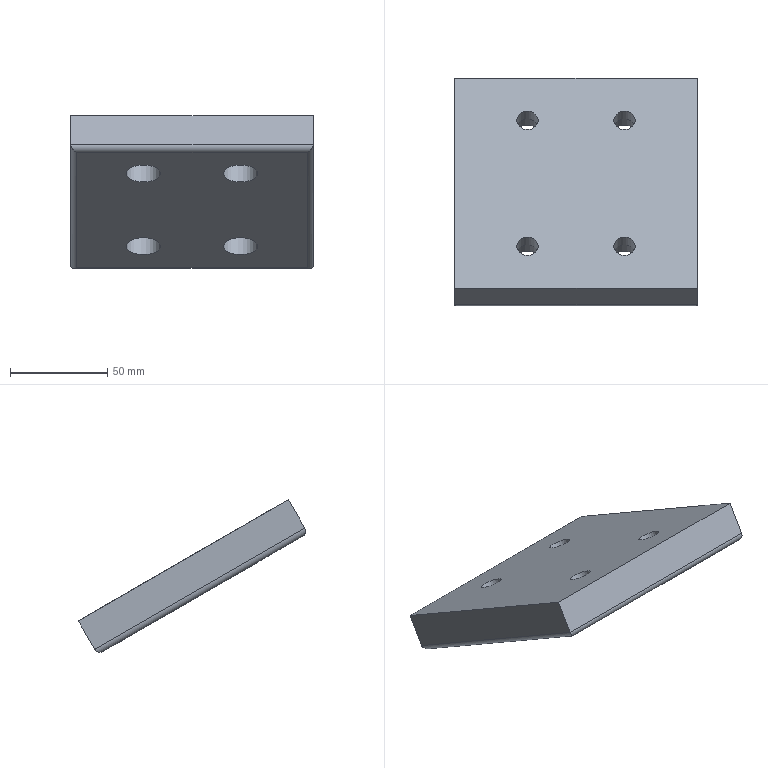Part | NX | features solid 2 | 1 solid | 22 faces | box 125 x 117.155 x 78.722 mm | volume 296958 mm3 | cylinder 12 | plane 10 | commonest cylinder face diameters 6 x4 11 x4 17.5 x4
STEP:
#1=CARTESIAN_POINT('',(605.,1052.897,-173.053));
#2=VERTEX_POINT('',#1);
#3=CARTESIAN_POINT('',(605.,1061.397,-158.331));
#4=VERTEX_POINT('',#3);
#5=CARTESIAN_POINT('',(605.,1051.397,-175.651));
#6=DIRECTION('',(0.,0.5,0.866));
#7=VECTOR('',#6,1000.);
#8=LINE('',#5,#7);
#9=EDGE_CURVE('',#2,#4,#8,.T.);
#10=ORIENTED_EDGE('',*,*,#9,.T.);
#11=CARTESIAN_POINT('',(605.,953.144,-95.831));
#12=VERTEX_POINT('',#11);
#13=CARTESIAN_POINT('',(605.,862.212,-43.331));
#14=DIRECTION('',(0.,-0.866,0.5));
#15=VECTOR('',#14,1000.);
#16=LINE('',#13,#15);
#17=EDGE_CURVE('',#4,#12,#16,.T.);
#18=ORIENTED_EDGE('',*,*,#17,.T.);
#19=CARTESIAN_POINT('',(605.,944.644,-110.553));
#20=VERTEX_POINT('',#19);
#21=CARTESIAN_POINT('',(605.,943.144,-113.151));
#22=DIRECTION('',(0.,-0.5,-0.866));
#23=VECTOR('',#22,1000.);
#24=LINE('',#21,#23);
#25=EDGE_CURVE('',#12,#20,#24,.T.);
#26=ORIENTED_EDGE('',*,*,#25,.T.);
#27=CARTESIAN_POINT('',(605.,944.644,-110.553));
#28=DIRECTION('',(0.,-0.866,0.5));
#29=VECTOR('',#28,1000.);
#30=LINE('',#27,#29);
#31=EDGE_CURVE('',#2,#20,#30,.T.);
#32=ORIENTED_EDGE('',*,*,#31,.F.);
#33=EDGE_LOOP('',(#10,#18,#26,#32));
#34=FACE_BOUND('',#33,.T.);
#35=CARTESIAN_POINT('',(605.,943.144,-113.151));
#36=DIRECTION('',(1.,0.,0.));
#37=DIRECTION('',(0.,0.5,0.866));
#38=AXIS2_PLACEMENT_3D('',#35,#36,#37);
#39=PLANE('',#38);
#40=ADVANCED_FACE('',(#34),#39,.T.);
#41=CARTESIAN_POINT('',(480.,944.644,-110.553));
#42=VERTEX_POINT('',#41);
#43=CARTESIAN_POINT('',(480.,953.144,-95.831));
#44=VERTEX_POINT('',#43);
#45=CARTESIAN_POINT('',(480.,943.144,-113.151));
#46=DIRECTION('',(0.,0.5,0.866));
#47=VECTOR('',#46,1000.);
#48=LINE('',#45,#47);
#49=EDGE_CURVE('',#42,#44,#48,.T.);
#50=ORIENTED_EDGE('',*,*,#49,.T.);
#51=CARTESIAN_POINT('',(480.,1061.397,-158.331));
#52=VERTEX_POINT('',#51);
#53=CARTESIAN_POINT('',(480.,862.212,-43.331));
#54=DIRECTION('',(0.,-0.866,0.5));
#55=VECTOR('',#54,1000.);
#56=LINE('',#53,#55);
#57=EDGE_CURVE('',#52,#44,#56,.T.);
#58=ORIENTED_EDGE('',*,*,#57,.F.);
#59=CARTESIAN_POINT('',(480.,1052.897,-173.053));
#60=VERTEX_POINT('',#59);
#61=CARTESIAN_POINT('',(480.,1051.397,-175.651));
#62=DIRECTION('',(0.,0.5,0.866));
#63=VECTOR('',#62,1000.);
#64=LINE('',#61,#63);
#65=EDGE_CURVE('',#60,#52,#64,.T.);
#66=ORIENTED_EDGE('',*,*,#65,.F.);
#67=CARTESIAN_POINT('',(480.,853.712,-58.053));
#68=DIRECTION('',(0.,-0.866,0.5));
#69=VECTOR('',#68,1000.);
#70=LINE('',#67,#69);
#71=EDGE_CURVE('',#42,#60,#70,.F.);
#72=ORIENTED_EDGE('',*,*,#71,.F.);
#73=EDGE_LOOP('',(#50,#58,#66,#72));
#74=FACE_BOUND('',#73,.T.);
#75=CARTESIAN_POINT('',(480.,852.212,-60.651));
#76=DIRECTION('',(1.,0.,0.));
#77=DIRECTION('',(0.,0.5,0.866));
#78=AXIS2_PLACEMENT_3D('',#75,#76,#77);
#79=PLANE('',#78);
#80=ADVANCED_FACE('',(#74),#79,.F.);
#81=CARTESIAN_POINT('',(558.75,1029.747,-163.151));
#82=VERTEX_POINT('',#81);
#83=CARTESIAN_POINT('',(567.5,1029.747,-163.151));
#84=DIRECTION('',(0.,0.5,0.866));
#85=DIRECTION('',(-1.,0.,0.));
#86=AXIS2_PLACEMENT_3D('',#83,#84,#85);
#87=CIRCLE('',#86,8.75);
#88=EDGE_CURVE('',#82,#82,#87,.T.);
#89=ORIENTED_EDGE('',*,*,#88,.T.);
#90=EDGE_LOOP('',(#89));
#91=FACE_BOUND('',#90,.T.);
#92=CARTESIAN_POINT('',(508.75,1029.747,-163.151));
#93=VERTEX_POINT('',#92);
#94=CARTESIAN_POINT('',(517.5,1029.747,-163.151));
#95=DIRECTION('',(0.,0.5,0.866));
#96=DIRECTION('',(-1.,0.,0.));
#97=AXIS2_PLACEMENT_3D('',#94,#95,#96);
#98=CIRCLE('',#97,8.75);
#99=EDGE_CURVE('',#93,#93,#98,.T.);
#100=ORIENTED_EDGE('',*,*,#99,.T.);
#101=EDGE_LOOP('',(#100));
#102=FACE_BOUND('',#101,.T.);
#103=CARTESIAN_POINT('',(558.75,964.795,-125.651));
#104=VERTEX_POINT('',#103);
#105=CARTESIAN_POINT('',(567.5,964.795,-125.651));
#106=DIRECTION('',(0.,0.5,0.866));
#107=DIRECTION('',(-1.,0.,0.));
#108=AXIS2_PLACEMENT_3D('',#105,#106,#107);
#109=CIRCLE('',#108,8.75);
#110=EDGE_CURVE('',#104,#104,#109,.T.);
#111=ORIENTED_EDGE('',*,*,#110,.T.);
#112=EDGE_LOOP('',(#111));
#113=FACE_BOUND('',#112,.T.);
#114=CARTESIAN_POINT('',(508.75,964.795,-125.651));
#115=VERTEX_POINT('',#114);
#116=CARTESIAN_POINT('',(517.5,964.795,-125.651));
#117=DIRECTION('',(0.,0.5,0.866));
#118=DIRECTION('',(-1.,0.,0.));
#119=AXIS2_PLACEMENT_3D('',#116,#117,#118);
#120=CIRCLE('',#119,8.75);
#121=EDGE_CURVE('',#115,#115,#120,.T.);
#122=ORIENTED_EDGE('',*,*,#121,.T.);
#123=EDGE_LOOP('',(#122));
#124=FACE_BOUND('',#123,.T.);
#125=CARTESIAN_POINT('',(602.,945.742,-114.651));
#126=VERTEX_POINT('',#125);
#127=CARTESIAN_POINT('',(602.,1048.799,-174.151));
#128=VERTEX_POINT('',#127);
#129=CARTESIAN_POINT('',(602.,1051.397,-175.651));
#130=DIRECTION('',(0.,-0.866,0.5));
#131=VECTOR('',#130,1000.);
#132=LINE('',#129,#131);
#133=EDGE_CURVE('',#126,#128,#132,.F.);
#134=ORIENTED_EDGE('',*,*,#133,.F.);
#135=CARTESIAN_POINT('',(483.,945.742,-114.651));
#136=VERTEX_POINT('',#135);
#137=CARTESIAN_POINT('',(483.,945.742,-114.651));
#138=DIRECTION('',(1.,0.,0.));
#139=VECTOR('',#138,1000.);
#140=LINE('',#137,#139);
#141=EDGE_CURVE('',#126,#136,#140,.F.);
#142=ORIENTED_EDGE('',*,*,#141,.T.);
#143=CARTESIAN_POINT('',(483.,1048.799,-174.151));
#144=VERTEX_POINT('',#143);
#145=CARTESIAN_POINT('',(483.,852.212,-60.651));
#146=DIRECTION('',(0.,-0.866,0.5));
#147=VECTOR('',#146,1000.);
#148=LINE('',#145,#147);
#149=EDGE_CURVE('',#144,#136,#148,.T.);
#150=ORIENTED_EDGE('',*,*,#149,.F.);
#151=CARTESIAN_POINT('',(480.,1048.799,-174.151));
#152=DIRECTION('',(1.,0.,0.));
#153=VECTOR('',#152,1000.);
#154=LINE('',#151,#153);
#155=EDGE_CURVE('',#128,#144,#154,.F.);
#156=ORIENTED_EDGE('',*,*,#155,.F.);
#157=EDGE_LOOP('',(#134,#142,#150,#156));
#158=FACE_BOUND('',#157,.T.);
#159=CARTESIAN_POINT('',(625.,852.212,-60.651));
#160=DIRECTION('',(0.,0.5,0.866));
#161=DIRECTION('',(1.,0.,0.));
#162=AXIS2_PLACEMENT_3D('',#159,#160,#161);
#163=PLANE('',#162);
#164=ADVANCED_FACE('',(#91,#102,#113,#124,#158),#163,.F.);
#165=CARTESIAN_POINT('',(562.,1039.747,-145.831));
#166=VERTEX_POINT('',#165);
#167=CARTESIAN_POINT('',(567.5,1039.747,-145.831));
#168=DIRECTION('',(0.,0.5,0.866));
#169=DIRECTION('',(-1.,0.,0.));
#170=AXIS2_PLACEMENT_3D('',#167,#168,#169);
#171=CIRCLE('',#170,5.5);
#172=EDGE_CURVE('',#166,#166,#171,.T.);
#173=ORIENTED_EDGE('',*,*,#172,.F.);
#174=EDGE_LOOP('',(#173));
#175=FACE_BOUND('',#174,.T.);
#176=CARTESIAN_POINT('',(512.,1039.747,-145.831));
#177=VERTEX_POINT('',#176);
#178=CARTESIAN_POINT('',(517.5,1039.747,-145.831));
#179=DIRECTION('',(0.,0.5,0.866));
#180=DIRECTION('',(-1.,0.,0.));
#181=AXIS2_PLACEMENT_3D('',#178,#179,#180);
#182=CIRCLE('',#181,5.5);
#183=EDGE_CURVE('',#177,#177,#182,.T.);
#184=ORIENTED_EDGE('',*,*,#183,.F.);
#185=EDGE_LOOP('',(#184));
#186=FACE_BOUND('',#185,.T.);
#187=CARTESIAN_POINT('',(562.,974.795,-108.331));
#188=VERTEX_POINT('',#187);
#189=CARTESIAN_POINT('',(567.5,974.795,-108.331));
#190=DIRECTION('',(0.,0.5,0.866));
#191=DIRECTION('',(-1.,0.,0.));
#192=AXIS2_PLACEMENT_3D('',#189,#190,#191);
#193=CIRCLE('',#192,5.5);
#194=EDGE_CURVE('',#188,#188,#193,.T.);
#195=ORIENTED_EDGE('',*,*,#194,.F.);
#196=EDGE_LOOP('',(#195));
#197=FACE_BOUND('',#196,.T.);
#198=CARTESIAN_POINT('',(512.,974.795,-108.331));
#199=VERTEX_POINT('',#198);
#200=CARTESIAN_POINT('',(517.5,974.795,-108.331));
#201=DIRECTION('',(0.,0.5,0.866));
#202=DIRECTION('',(-1.,0.,0.));
#203=AXIS2_PLACEMENT_3D('',#200,#201,#202);
#204=CIRCLE('',#203,5.5);
#205=EDGE_CURVE('',#199,#199,#204,.T.);
#206=ORIENTED_EDGE('',*,*,#205,.F.);
#207=EDGE_LOOP('',(#206));
#208=FACE_BOUND('',#207,.T.);
#209=CARTESIAN_POINT('',(470.,1061.397,-158.331));
#210=DIRECTION('',(1.,0.,0.));
#211=VECTOR('',#210,1000.);
#212=LINE('',#209,#211);
#213=EDGE_CURVE('',#52,#4,#212,.T.);
#214=ORIENTED_EDGE('',*,*,#213,.F.);
#215=ORIENTED_EDGE('',*,*,#57,.T.);
#216=CARTESIAN_POINT('',(730.,953.144,-95.831));
#217=DIRECTION('',(-1.,0.,0.));
#218=VECTOR('',#217,1000.);
#219=LINE('',#216,#218);
#220=EDGE_CURVE('',#12,#44,#219,.T.);
#221=ORIENTED_EDGE('',*,*,#220,.F.);
#222=ORIENTED_EDGE('',*,*,#17,.F.);
#223=EDGE_LOOP('',(#214,#215,#221,#222));
#224=FACE_BOUND('',#223,.T.);
#225=CARTESIAN_POINT('',(625.,862.212,-43.331));
#226=DIRECTION('',(0.,0.5,0.866));
#227=DIRECTION('',(1.,0.,0.));
#228=AXIS2_PLACEMENT_3D('',#225,#226,#227);
#229=PLANE('',#228);
#230=ADVANCED_FACE('',(#175,#186,#197,#208,#224),#229,.T.);
#231=ORIENTED_EDGE('',*,*,#65,.T.);
#232=ORIENTED_EDGE('',*,*,#213,.T.);
#233=ORIENTED_EDGE('',*,*,#9,.F.);
#234=CARTESIAN_POINT('',(605.,1052.897,-173.053));
#235=DIRECTION('',(1.,0.,0.));
#236=VECTOR('',#235,1000.);
#237=LINE('',#234,#236);
#238=EDGE_CURVE('',#60,#2,#237,.T.);
#239=ORIENTED_EDGE('',*,*,#238,.F.);
#240=EDGE_LOOP('',(#231,#232,#233,#239));
#241=FACE_BOUND('',#240,.T.);
#242=CARTESIAN_POINT('',(470.,1051.397,-175.651));
#243=DIRECTION('',(0.,0.866,-0.5));
#244=DIRECTION('',(0.866,0.25,0.433));
#245=AXIS2_PLACEMENT_3D('',#242,#243,#244);
#246=PLANE('',#245);
#247=ADVANCED_FACE('',(#241),#246,.T.);
#248=ORIENTED_EDGE('',*,*,#49,.F.);
#249=CARTESIAN_POINT('',(602.,944.644,-110.553));
#250=DIRECTION('',(1.,0.,0.));
#251=VECTOR('',#250,1000.);
#252=LINE('',#249,#251);
#253=EDGE_CURVE('',#42,#20,#252,.T.);
#254=ORIENTED_EDGE('',*,*,#253,.T.);
#255=ORIENTED_EDGE('',*,*,#25,.F.);
#256=ORIENTED_EDGE('',*,*,#220,.T.);
#257=EDGE_LOOP('',(#248,#254,#255,#256));
#258=FACE_BOUND('',#257,.T.);
#259=CARTESIAN_POINT('',(730.,943.144,-113.151));
#260=DIRECTION('',(0.,-0.866,0.5));
#261=DIRECTION('',(-0.866,-0.25,-0.433));
#262=AXIS2_PLACEMENT_3D('',#259,#260,#261);
#263=PLANE('',#262);
#264=ADVANCED_FACE('',(#258),#263,.T.);
#265=ORIENTED_EDGE('',*,*,#149,.T.);
#266=CARTESIAN_POINT('',(483.,947.242,-112.053));
#267=DIRECTION('',(0.7071,-0.6124,0.3536));
#268=DIRECTION('',(-0.7071,-0.6124,0.3536));
#269=AXIS2_PLACEMENT_3D('',#266,#267,#268);
#270=ELLIPSE('',#269,4.243,3.);
#271=EDGE_CURVE('',#136,#42,#270,.F.);
#272=ORIENTED_EDGE('',*,*,#271,.T.);
#273=ORIENTED_EDGE('',*,*,#71,.T.);
#274=CARTESIAN_POINT('',(483.,1050.299,-171.553));
#275=DIRECTION('',(0.7071,0.6124,-0.3536));
#276=DIRECTION('',(0.7071,-0.6124,0.3536));
#277=AXIS2_PLACEMENT_3D('',#274,#275,#276);
#278=ELLIPSE('',#277,4.243,3.);
#279=EDGE_CURVE('',#60,#144,#278,.F.);
#280=ORIENTED_EDGE('',*,*,#279,.T.);
#281=EDGE_LOOP('',(#265,#272,#273,#280));
#282=FACE_BOUND('',#281,.T.);
#283=CARTESIAN_POINT('',(483.,853.712,-58.053));
#284=DIRECTION('',(0.,-0.866,0.5));
#285=DIRECTION('',(-0.5,0.433,0.75));
#286=AXIS2_PLACEMENT_3D('',#283,#284,#285);
#287=CYLINDRICAL_SURFACE('',#286,3.);
#288=ADVANCED_FACE('',(#282),#287,.T.);
#289=ORIENTED_EDGE('',*,*,#31,.T.);
#290=CARTESIAN_POINT('',(602.,947.242,-112.053));
#291=DIRECTION('',(0.7071,0.6124,-0.3536));
#292=DIRECTION('',(-0.7071,0.6124,-0.3536));
#293=AXIS2_PLACEMENT_3D('',#290,#291,#292);
#294=ELLIPSE('',#293,4.243,3.);
#295=EDGE_CURVE('',#20,#126,#294,.T.);
#296=ORIENTED_EDGE('',*,*,#295,.T.);
#297=ORIENTED_EDGE('',*,*,#133,.T.);
#298=CARTESIAN_POINT('',(602.,1050.299,-171.553));
#299=DIRECTION('',(0.7071,-0.6124,0.3536));
#300=DIRECTION('',(0.7071,0.6124,-0.3536));
#301=AXIS2_PLACEMENT_3D('',#298,#299,#300);
#302=ELLIPSE('',#301,4.243,3.);
#303=EDGE_CURVE('',#128,#2,#302,.T.);
#304=ORIENTED_EDGE('',*,*,#303,.T.);
#305=EDGE_LOOP('',(#289,#296,#297,#304));
#306=FACE_BOUND('',#305,.T.);
#307=CARTESIAN_POINT('',(602.,944.644,-110.553));
#308=DIRECTION('',(0.,0.866,-0.5));
#309=DIRECTION('',(0.5,-0.433,-0.75));
#310=AXIS2_PLACEMENT_3D('',#307,#308,#309);
#311=CYLINDRICAL_SURFACE('',#310,3.);
#312=ADVANCED_FACE('',(#306),#311,.T.);
#313=ORIENTED_EDGE('',*,*,#279,.F.);
#314=ORIENTED_EDGE('',*,*,#238,.T.);
#315=ORIENTED_EDGE('',*,*,#303,.F.);
#316=ORIENTED_EDGE('',*,*,#155,.T.);
#317=EDGE_LOOP('',(#313,#314,#315,#316));
#318=FACE_BOUND('',#317,.T.);
#319=CARTESIAN_POINT('',(470.,1050.299,-171.553));
#320=DIRECTION('',(-1.,0.,0.));
#321=DIRECTION('',(0.,-0.5,-0.866));
#322=AXIS2_PLACEMENT_3D('',#319,#320,#321);
#323=CYLINDRICAL_SURFACE('',#322,3.);
#324=ADVANCED_FACE('',(#318),#323,.T.);
#325=ORIENTED_EDGE('',*,*,#271,.F.);
#326=ORIENTED_EDGE('',*,*,#141,.F.);
#327=ORIENTED_EDGE('',*,*,#295,.F.);
#328=ORIENTED_EDGE('',*,*,#253,.F.);
#329=EDGE_LOOP('',(#325,#326,#327,#328));
#330=FACE_BOUND('',#329,.T.);
#331=CARTESIAN_POINT('',(730.,947.242,-112.053));
#332=DIRECTION('',(-1.,0.,0.));
#333=DIRECTION('',(0.,-0.5,-0.866));
#334=AXIS2_PLACEMENT_3D('',#331,#332,#333);
#335=CYLINDRICAL_SURFACE('',#334,3.);
#336=ADVANCED_FACE('',(#330),#335,.T.);
#337=ORIENTED_EDGE('',*,*,#205,.T.);
#338=EDGE_LOOP('',(#337));
#339=FACE_BOUND('',#338,.T.);
#340=CARTESIAN_POINT('',(512.,970.795,-115.259));
#341=VERTEX_POINT('',#340);
#342=CARTESIAN_POINT('',(517.5,970.795,-115.259));
#343=DIRECTION('',(0.,0.5,0.866));
#344=DIRECTION('',(-1.,0.,0.));
#345=AXIS2_PLACEMENT_3D('',#342,#343,#344);
#346=CIRCLE('',#345,5.5);
#347=EDGE_CURVE('',#341,#341,#346,.T.);
#348=ORIENTED_EDGE('',*,*,#347,.F.);
#349=EDGE_LOOP('',(#348));
#350=FACE_BOUND('',#349,.T.);
#351=CARTESIAN_POINT('',(517.5,1014.795,-39.049));
#352=DIRECTION('',(0.,0.5,0.866));
#353=DIRECTION('',(-1.,0.,0.));
#354=AXIS2_PLACEMENT_3D('',#351,#352,#353);
#355=CYLINDRICAL_SURFACE('',#354,5.5);
#356=ADVANCED_FACE('',(#339,#350),#355,.F.);
#357=ORIENTED_EDGE('',*,*,#347,.T.);
#358=EDGE_LOOP('',(#357));
#359=FACE_BOUND('',#358,.T.);
#360=CARTESIAN_POINT('',(508.75,970.795,-115.259));
#361=VERTEX_POINT('',#360);
#362=CARTESIAN_POINT('',(517.5,970.795,-115.259));
#363=DIRECTION('',(0.,0.5,0.866));
#364=DIRECTION('',(-1.,0.,0.));
#365=AXIS2_PLACEMENT_3D('',#362,#363,#364);
#366=CIRCLE('',#365,8.75);
#367=EDGE_CURVE('',#361,#361,#366,.T.);
#368=ORIENTED_EDGE('',*,*,#367,.F.);
#369=EDGE_LOOP('',(#368));
#370=FACE_BOUND('',#369,.T.);
#371=CARTESIAN_POINT('',(517.5,970.795,-115.259));
#372=DIRECTION('',(0.,0.5,0.866));
#373=DIRECTION('',(-1.,0.,0.));
#374=AXIS2_PLACEMENT_3D('',#371,#372,#373);
#375=PLANE('',#374);
#376=ADVANCED_FACE('',(#359,#370),#375,.F.);
#377=ORIENTED_EDGE('',*,*,#367,.T.);
#378=EDGE_LOOP('',(#377));
#379=FACE_BOUND('',#378,.T.);
#380=ORIENTED_EDGE('',*,*,#121,.F.);
#381=EDGE_LOOP('',(#380));
#382=FACE_BOUND('',#381,.T.);
#383=CARTESIAN_POINT('',(517.5,964.795,-125.651));
#384=DIRECTION('',(0.,0.5,0.866));
#385=DIRECTION('',(-1.,0.,0.));
#386=AXIS2_PLACEMENT_3D('',#383,#384,#385);
#387=CYLINDRICAL_SURFACE('',#386,8.75);
#388=ADVANCED_FACE('',(#379,#382),#387,.F.);
#389=ORIENTED_EDGE('',*,*,#194,.T.);
#390=EDGE_LOOP('',(#389));
#391=FACE_BOUND('',#390,.T.);
#392=CARTESIAN_POINT('',(562.,970.795,-115.259));
#393=VERTEX_POINT('',#392);
#394=CARTESIAN_POINT('',(567.5,970.795,-115.259));
#395=DIRECTION('',(0.,0.5,0.866));
#396=DIRECTION('',(-1.,0.,0.));
#397=AXIS2_PLACEMENT_3D('',#394,#395,#396);
#398=CIRCLE('',#397,5.5);
#399=EDGE_CURVE('',#393,#393,#398,.T.);
#400=ORIENTED_EDGE('',*,*,#399,.F.);
#401=EDGE_LOOP('',(#400));
#402=FACE_BOUND('',#401,.T.);
#403=CARTESIAN_POINT('',(567.5,1014.795,-39.049));
#404=DIRECTION('',(0.,0.5,0.866));
#405=DIRECTION('',(-1.,0.,0.));
#406=AXIS2_PLACEMENT_3D('',#403,#404,#405);
#407=CYLINDRICAL_SURFACE('',#406,5.5);
#408=ADVANCED_FACE('',(#391,#402),#407,.F.);
#409=ORIENTED_EDGE('',*,*,#399,.T.);
#410=EDGE_LOOP('',(#409));
#411=FACE_BOUND('',#410,.T.);
#412=CARTESIAN_POINT('',(558.75,970.795,-115.259));
#413=VERTEX_POINT('',#412);
#414=CARTESIAN_POINT('',(567.5,970.795,-115.259));
#415=DIRECTION('',(0.,0.5,0.866));
#416=DIRECTION('',(-1.,0.,0.));
#417=AXIS2_PLACEMENT_3D('',#414,#415,#416);
#418=CIRCLE('',#417,8.75);
#419=EDGE_CURVE('',#413,#413,#418,.T.);
#420=ORIENTED_EDGE('',*,*,#419,.F.);
#421=EDGE_LOOP('',(#420));
#422=FACE_BOUND('',#421,.T.);
#423=CARTESIAN_POINT('',(567.5,970.795,-115.259));
#424=DIRECTION('',(0.,0.5,0.866));
#425=DIRECTION('',(-1.,0.,0.));
#426=AXIS2_PLACEMENT_3D('',#423,#424,#425);
#427=PLANE('',#426);
#428=ADVANCED_FACE('',(#411,#422),#427,.F.);
#429=ORIENTED_EDGE('',*,*,#419,.T.);
#430=EDGE_LOOP('',(#429));
#431=FACE_BOUND('',#430,.T.);
#432=ORIENTED_EDGE('',*,*,#110,.F.);
#433=EDGE_LOOP('',(#432));
#434=FACE_BOUND('',#433,.T.);
#435=CARTESIAN_POINT('',(567.5,964.795,-125.651));
#436=DIRECTION('',(0.,0.5,0.866));
#437=DIRECTION('',(-1.,0.,0.));
#438=AXIS2_PLACEMENT_3D('',#435,#436,#437);
#439=CYLINDRICAL_SURFACE('',#438,8.75);
#440=ADVANCED_FACE('',(#431,#434),#439,.F.);
#441=ORIENTED_EDGE('',*,*,#183,.T.);
#442=EDGE_LOOP('',(#441));
#443=FACE_BOUND('',#442,.T.);
#444=CARTESIAN_POINT('',(512.,1035.747,-152.759));
#445=VERTEX_POINT('',#444);
#446=CARTESIAN_POINT('',(517.5,1035.747,-152.759));
#447=DIRECTION('',(0.,0.5,0.866));
#448=DIRECTION('',(-1.,0.,0.));
#449=AXIS2_PLACEMENT_3D('',#446,#447,#448);
#450=CIRCLE('',#449,5.5);
#451=EDGE_CURVE('',#445,#445,#450,.T.);
#452=ORIENTED_EDGE('',*,*,#451,.F.);
#453=EDGE_LOOP('',(#452));
#454=FACE_BOUND('',#453,.T.);
#455=CARTESIAN_POINT('',(517.5,1079.747,-76.549));
#456=DIRECTION('',(0.,0.5,0.866));
#457=DIRECTION('',(-1.,0.,0.));
#458=AXIS2_PLACEMENT_3D('',#455,#456,#457);
#459=CYLINDRICAL_SURFACE('',#458,5.5);
#460=ADVANCED_FACE('',(#443,#454),#459,.F.);
#461=ORIENTED_EDGE('',*,*,#451,.T.);
#462=EDGE_LOOP('',(#461));
#463=FACE_BOUND('',#462,.T.);
#464=CARTESIAN_POINT('',(508.75,1035.747,-152.759));
#465=VERTEX_POINT('',#464);
#466=CARTESIAN_POINT('',(517.5,1035.747,-152.759));
#467=DIRECTION('',(0.,0.5,0.866));
#468=DIRECTION('',(-1.,0.,0.));
#469=AXIS2_PLACEMENT_3D('',#466,#467,#468);
#470=CIRCLE('',#469,8.75);
#471=EDGE_CURVE('',#465,#465,#470,.T.);
#472=ORIENTED_EDGE('',*,*,#471,.F.);
#473=EDGE_LOOP('',(#472));
#474=FACE_BOUND('',#473,.T.);
#475=CARTESIAN_POINT('',(517.5,1035.747,-152.759));
#476=DIRECTION('',(0.,0.5,0.866));
#477=DIRECTION('',(-1.,0.,0.));
#478=AXIS2_PLACEMENT_3D('',#475,#476,#477);
#479=PLANE('',#478);
#480=ADVANCED_FACE('',(#463,#474),#479,.F.);
#481=ORIENTED_EDGE('',*,*,#471,.T.);
#482=EDGE_LOOP('',(#481));
#483=FACE_BOUND('',#482,.T.);
#484=ORIENTED_EDGE('',*,*,#99,.F.);
#485=EDGE_LOOP('',(#484));
#486=FACE_BOUND('',#485,.T.);
#487=CARTESIAN_POINT('',(517.5,1029.747,-163.151));
#488=DIRECTION('',(0.,0.5,0.866));
#489=DIRECTION('',(-1.,0.,0.));
#490=AXIS2_PLACEMENT_3D('',#487,#488,#489);
#491=CYLINDRICAL_SURFACE('',#490,8.75);
#492=ADVANCED_FACE('',(#483,#486),#491,.F.);
#493=ORIENTED_EDGE('',*,*,#172,.T.);
#494=EDGE_LOOP('',(#493));
#495=FACE_BOUND('',#494,.T.);
#496=CARTESIAN_POINT('',(562.,1035.747,-152.759));
#497=VERTEX_POINT('',#496);
#498=CARTESIAN_POINT('',(567.5,1035.747,-152.759));
#499=DIRECTION('',(0.,0.5,0.866));
#500=DIRECTION('',(-1.,0.,0.));
#501=AXIS2_PLACEMENT_3D('',#498,#499,#500);
#502=CIRCLE('',#501,5.5);
#503=EDGE_CURVE('',#497,#497,#502,.T.);
#504=ORIENTED_EDGE('',*,*,#503,.F.);
#505=EDGE_LOOP('',(#504));
#506=FACE_BOUND('',#505,.T.);
#507=CARTESIAN_POINT('',(567.5,1079.747,-76.549));
#508=DIRECTION('',(0.,0.5,0.866));
#509=DIRECTION('',(-1.,0.,0.));
#510=AXIS2_PLACEMENT_3D('',#507,#508,#509);
#511=CYLINDRICAL_SURFACE('',#510,5.5);
#512=ADVANCED_FACE('',(#495,#506),#511,.F.);
#513=ORIENTED_EDGE('',*,*,#503,.T.);
#514=EDGE_LOOP('',(#513));
#515=FACE_BOUND('',#514,.T.);
#516=CARTESIAN_POINT('',(558.75,1035.747,-152.759));
#517=VERTEX_POINT('',#516);
#518=CARTESIAN_POINT('',(567.5,1035.747,-152.759));
#519=DIRECTION('',(0.,0.5,0.866));
#520=DIRECTION('',(-1.,0.,0.));
#521=AXIS2_PLACEMENT_3D('',#518,#519,#520);
#522=CIRCLE('',#521,8.75);
#523=EDGE_CURVE('',#517,#517,#522,.T.);
#524=ORIENTED_EDGE('',*,*,#523,.F.);
#525=EDGE_LOOP('',(#524));
#526=FACE_BOUND('',#525,.T.);
#527=CARTESIAN_POINT('',(567.5,1035.747,-152.759));
#528=DIRECTION('',(0.,0.5,0.866));
#529=DIRECTION('',(-1.,0.,0.));
#530=AXIS2_PLACEMENT_3D('',#527,#528,#529);
#531=PLANE('',#530);
#532=ADVANCED_FACE('',(#515,#526),#531,.F.);
#533=ORIENTED_EDGE('',*,*,#523,.T.);
#534=EDGE_LOOP('',(#533));
#535=FACE_BOUND('',#534,.T.);
#536=ORIENTED_EDGE('',*,*,#88,.F.);
#537=EDGE_LOOP('',(#536));
#538=FACE_BOUND('',#537,.T.);
#539=CARTESIAN_POINT('',(567.5,1029.747,-163.151));
#540=DIRECTION('',(0.,0.5,0.866));
#541=DIRECTION('',(-1.,0.,0.));
#542=AXIS2_PLACEMENT_3D('',#539,#540,#541);
#543=CYLINDRICAL_SURFACE('',#542,8.75);
#544=ADVANCED_FACE('',(#535,#538),#543,.F.);
#545=CLOSED_SHELL('',(#40,#80,#164,#230,#247,#264,#288,#312,#324,#336,#356,#376,#388,#408,#428,#440,#460,#480,#492,#512,#532,#544));
#546=MANIFOLD_SOLID_BREP('',#545);
#547=(LENGTH_UNIT()NAMED_UNIT(*)SI_UNIT(.MILLI.,.METRE.));
#548=UNCERTAINTY_MEASURE_WITH_UNIT(LENGTH_MEASURE(0.00001),#547,'','');
#549=(NAMED_UNIT(*)PLANE_ANGLE_UNIT()SI_UNIT($,.RADIAN.));
#550=(NAMED_UNIT(*)SI_UNIT($,.STERADIAN.)SOLID_ANGLE_UNIT());
#551=(GEOMETRIC_REPRESENTATION_CONTEXT(3)GLOBAL_UNCERTAINTY_ASSIGNED_CONTEXT((#548))GLOBAL_UNIT_ASSIGNED_CONTEXT((#547,#549,#550))REPRESENTATION_CONTEXT('',''));
#552=ADVANCED_BREP_SHAPE_REPRESENTATION('',(#546),#551);